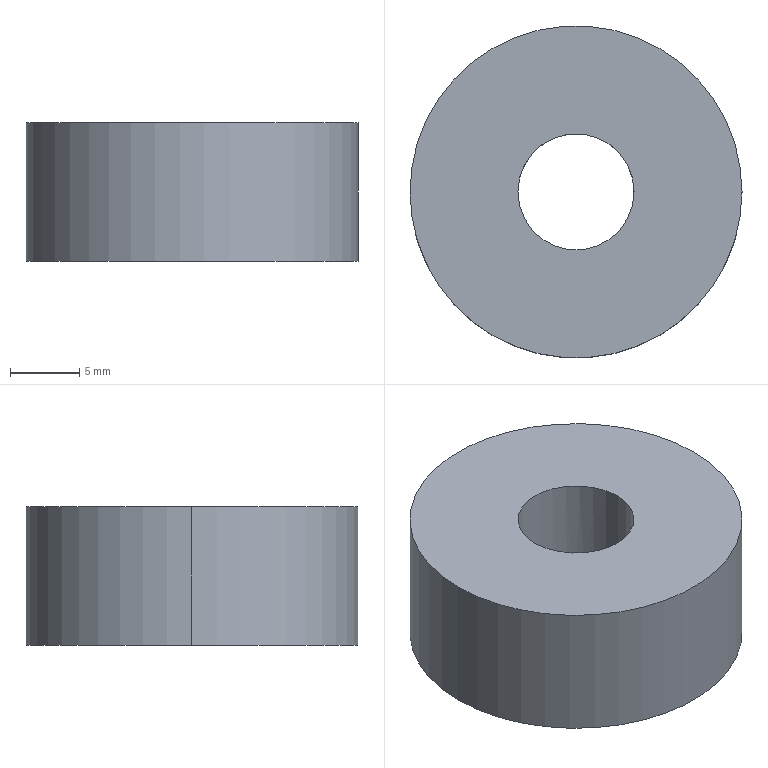Part | STEP file | PN_0033_Default<As Machined> | 1 solid | 6 faces | box 24 x 24 x 10 mm | volume 3970 mm3 | cylinder 4 | plane 2 | commonest cylinder face diameters 8.4 x2 24 x2
STEP:
#1=CARTESIAN_POINT('',(-4.2,0.,-10.));
#2=VERTEX_POINT('',#1);
#3=CARTESIAN_POINT('',(4.2,0.,-10.));
#4=VERTEX_POINT('',#3);
#5=CARTESIAN_POINT('',(0.,0.,-10.));
#6=DIRECTION('',(0.,0.,1.));
#7=AXIS2_PLACEMENT_3D('',#5,#6,$);
#8=CIRCLE('',#7,4.2);
#9=EDGE_CURVE('',#2,#4,#8,.T.);
#10=ORIENTED_EDGE('',*,*,#9,.F.);
#11=CARTESIAN_POINT('',(-4.2,0.,0.));
#12=VERTEX_POINT('',#11);
#13=CARTESIAN_POINT('',(-4.2,0.,-2.));
#14=DIRECTION('',(0.,0.,1.));
#15=VECTOR('',#14,1.);
#16=LINE('',#13,#15);
#17=EDGE_CURVE('',#2,#12,#16,.T.);
#18=ORIENTED_EDGE('',*,*,#17,.T.);
#19=CARTESIAN_POINT('',(4.2,0.,0.));
#20=VERTEX_POINT('',#19);
#21=CARTESIAN_POINT('',(0.,0.,0.));
#22=DIRECTION('',(0.,0.,1.));
#23=AXIS2_PLACEMENT_3D('',#21,#22,$);
#24=CIRCLE('',#23,4.2);
#25=EDGE_CURVE('',#12,#20,#24,.T.);
#26=ORIENTED_EDGE('',*,*,#25,.T.);
#27=CARTESIAN_POINT('',(4.2,0.,-2.));
#28=DIRECTION('',(0.,0.,1.));
#29=VECTOR('',#28,1.);
#30=LINE('',#27,#29);
#31=EDGE_CURVE('',#4,#20,#30,.T.);
#32=ORIENTED_EDGE('',*,*,#31,.F.);
#33=EDGE_LOOP('',(#10,#18,#26,#32));
#34=FACE_OUTER_BOUND('',#33,.T.);
#35=CARTESIAN_POINT('',(0.,0.,-2.));
#36=DIRECTION('',(0.,0.,1.));
#37=DIRECTION('',(-1.,0.,0.));
#38=AXIS2_PLACEMENT_3D('',#35,#36,#37);
#39=CYLINDRICAL_SURFACE('',#38,4.2);
#40=ADVANCED_FACE('',(#34),#39,.F.);
#41=CARTESIAN_POINT('',(12.,0.,-10.));
#42=VERTEX_POINT('',#41);
#43=CARTESIAN_POINT('',(-12.,0.,-10.));
#44=VERTEX_POINT('',#43);
#45=CARTESIAN_POINT('',(0.,0.,-10.));
#46=DIRECTION('',(0.,0.,-1.));
#47=AXIS2_PLACEMENT_3D('',#45,#46,$);
#48=CIRCLE('',#47,12.);
#49=EDGE_CURVE('',#42,#44,#48,.T.);
#50=ORIENTED_EDGE('',*,*,#49,.T.);
#51=CARTESIAN_POINT('',(0.,0.,-10.));
#52=DIRECTION('',(0.,0.,-1.));
#53=AXIS2_PLACEMENT_3D('',#51,#52,$);
#54=CIRCLE('',#53,12.);
#55=EDGE_CURVE('',#44,#42,#54,.T.);
#56=ORIENTED_EDGE('',*,*,#55,.T.);
#57=EDGE_LOOP('',(#50,#56));
#58=FACE_OUTER_BOUND('',#57,.T.);
#59=CARTESIAN_POINT('',(4.2,0.,-10.));
#60=CARTESIAN_POINT('',(4.2,0.4016,-10.));
#61=CARTESIAN_POINT('',(4.152,0.8032,-10.));
#62=CARTESIAN_POINT('',(4.056,1.197,-10.));
#63=CARTESIAN_POINT('',(3.772,1.954,-10.));
#64=CARTESIAN_POINT('',(3.317,2.623,-10.));
#65=CARTESIAN_POINT('',(3.05,2.929,-10.));
#66=CARTESIAN_POINT('',(2.45,3.471,-10.));
#67=CARTESIAN_POINT('',(1.738,3.855,-10.));
#68=CARTESIAN_POINT('',(1.361,4.004,-10.));
#69=CARTESIAN_POINT('',(0.5781,4.208,-10.));
#70=CARTESIAN_POINT('',(-0.2306,4.223,-10.));
#71=CARTESIAN_POINT('',(-0.634,4.181,-10.));
#72=CARTESIAN_POINT('',(-1.423,4.003,-10.));
#73=CARTESIAN_POINT('',(-2.148,3.643,-10.));
#74=CARTESIAN_POINT('',(-2.487,3.421,-10.));
#75=CARTESIAN_POINT('',(-3.105,2.899,-10.));
#76=CARTESIAN_POINT('',(-3.583,2.247,-10.));
#77=CARTESIAN_POINT('',(-3.782,1.893,-10.));
#78=CARTESIAN_POINT('',(-4.024,1.306,-10.));
#79=CARTESIAN_POINT('',(-4.153,0.6866,-10.));
#80=CARTESIAN_POINT('',(-4.184,0.4587,-10.));
#81=CARTESIAN_POINT('',(-4.2,0.2294,-10.));
#82=CARTESIAN_POINT('',(-4.2,0.,-10.));
#83=B_SPLINE_CURVE_WITH_KNOTS('',5,(#59,#60,#61,#62,#63,#64,#65,#66,#67,#68,#69,#70,#71,#72,#73,#74,#75,#76,#77,#78,#79,#80,#81,#82),.UNSPECIFIED.,.F.,.U.,(6,3,3,3,3,3,3,6),(0.,2.84,5.679,8.519,11.359,14.198,17.038,18.66),.UNSPECIFIED.);
#84=EDGE_CURVE('',#4,#2,#83,.T.);
#85=ORIENTED_EDGE('',*,*,#84,.T.);
#86=ORIENTED_EDGE('',*,*,#9,.T.);
#87=EDGE_LOOP('',(#85,#86));
#88=FACE_BOUND('',#87,.T.);
#89=CARTESIAN_POINT('',(0.,0.,-10.));
#90=DIRECTION('',(0.,0.,-1.));
#91=DIRECTION('',(-1.,0.,0.));
#92=AXIS2_PLACEMENT_3D('',#89,#90,#91);
#93=PLANE('',#92);
#94=ADVANCED_FACE('',(#58,#88),#93,.T.);
#95=ORIENTED_EDGE('',*,*,#17,.F.);
#96=ORIENTED_EDGE('',*,*,#84,.F.);
#97=ORIENTED_EDGE('',*,*,#31,.T.);
#98=CARTESIAN_POINT('',(0.,0.,0.));
#99=DIRECTION('',(0.,0.,1.));
#100=AXIS2_PLACEMENT_3D('',#98,#99,$);
#101=CIRCLE('',#100,4.2);
#102=EDGE_CURVE('',#20,#12,#101,.T.);
#103=ORIENTED_EDGE('',*,*,#102,.T.);
#104=EDGE_LOOP('',(#95,#96,#97,#103));
#105=FACE_OUTER_BOUND('',#104,.T.);
#106=CARTESIAN_POINT('',(0.,0.,-2.));
#107=DIRECTION('',(0.,0.,1.));
#108=DIRECTION('',(1.,0.,0.));
#109=AXIS2_PLACEMENT_3D('',#106,#107,#108);
#110=CYLINDRICAL_SURFACE('',#109,4.2);
#111=ADVANCED_FACE('',(#105),#110,.F.);
#112=CARTESIAN_POINT('',(12.,0.,0.));
#113=VERTEX_POINT('',#112);
#114=CARTESIAN_POINT('',(-12.,0.,0.));
#115=VERTEX_POINT('',#114);
#116=CARTESIAN_POINT('',(0.,0.,0.));
#117=DIRECTION('',(0.,0.,1.));
#118=AXIS2_PLACEMENT_3D('',#116,#117,$);
#119=CIRCLE('',#118,12.);
#120=EDGE_CURVE('',#113,#115,#119,.T.);
#121=ORIENTED_EDGE('',*,*,#120,.T.);
#122=CARTESIAN_POINT('',(0.,0.,0.));
#123=DIRECTION('',(0.,0.,1.));
#124=AXIS2_PLACEMENT_3D('',#122,#123,$);
#125=CIRCLE('',#124,12.);
#126=EDGE_CURVE('',#115,#113,#125,.T.);
#127=ORIENTED_EDGE('',*,*,#126,.T.);
#128=EDGE_LOOP('',(#121,#127));
#129=FACE_OUTER_BOUND('',#128,.T.);
#130=ORIENTED_EDGE('',*,*,#102,.F.);
#131=ORIENTED_EDGE('',*,*,#25,.F.);
#132=EDGE_LOOP('',(#130,#131));
#133=FACE_BOUND('',#132,.T.);
#134=CARTESIAN_POINT('',(0.,0.,0.));
#135=DIRECTION('',(0.,0.,1.));
#136=DIRECTION('',(1.,0.,0.));
#137=AXIS2_PLACEMENT_3D('',#134,#135,#136);
#138=PLANE('',#137);
#139=ADVANCED_FACE('',(#129,#133),#138,.T.);
#140=CARTESIAN_POINT('',(-12.,0.,-2.));
#141=DIRECTION('',(0.,0.,1.));
#142=VECTOR('',#141,1.);
#143=LINE('',#140,#142);
#144=EDGE_CURVE('',#44,#115,#143,.T.);
#145=ORIENTED_EDGE('',*,*,#144,.F.);
#146=ORIENTED_EDGE('',*,*,#49,.F.);
#147=CARTESIAN_POINT('',(12.,0.,-2.));
#148=DIRECTION('',(0.,0.,1.));
#149=VECTOR('',#148,1.);
#150=LINE('',#147,#149);
#151=EDGE_CURVE('',#42,#113,#150,.T.);
#152=ORIENTED_EDGE('',*,*,#151,.T.);
#153=ORIENTED_EDGE('',*,*,#126,.F.);
#154=EDGE_LOOP('',(#145,#146,#152,#153));
#155=FACE_OUTER_BOUND('',#154,.T.);
#156=CARTESIAN_POINT('',(0.,0.,-2.));
#157=DIRECTION('',(0.,0.,1.));
#158=DIRECTION('',(-1.,0.,0.));
#159=AXIS2_PLACEMENT_3D('',#156,#157,#158);
#160=CYLINDRICAL_SURFACE('',#159,12.);
#161=ADVANCED_FACE('',(#155),#160,.T.);
#162=ORIENTED_EDGE('',*,*,#55,.F.);
#163=ORIENTED_EDGE('',*,*,#144,.T.);
#164=ORIENTED_EDGE('',*,*,#120,.F.);
#165=ORIENTED_EDGE('',*,*,#151,.F.);
#166=EDGE_LOOP('',(#162,#163,#164,#165));
#167=FACE_OUTER_BOUND('',#166,.T.);
#168=CARTESIAN_POINT('',(0.,0.,-2.));
#169=DIRECTION('',(0.,0.,1.));
#170=DIRECTION('',(1.,0.,0.));
#171=AXIS2_PLACEMENT_3D('',#168,#169,#170);
#172=CYLINDRICAL_SURFACE('',#171,12.);
#173=ADVANCED_FACE('',(#167),#172,.T.);
#174=CLOSED_SHELL('',(#40,#94,#111,#139,#161,#173));
#175=MANIFOLD_SOLID_BREP('',#174);
#176=(LENGTH_UNIT()NAMED_UNIT(*)SI_UNIT(.MILLI.,.METRE.));
#177=UNCERTAINTY_MEASURE_WITH_UNIT(LENGTH_MEASURE(0.005),#176,'','');
#178=(NAMED_UNIT(*)PLANE_ANGLE_UNIT()SI_UNIT($,.RADIAN.));
#179=(NAMED_UNIT(*)SI_UNIT($,.STERADIAN.)SOLID_ANGLE_UNIT());
#180=(GEOMETRIC_REPRESENTATION_CONTEXT(3)GLOBAL_UNCERTAINTY_ASSIGNED_CONTEXT((#177))GLOBAL_UNIT_ASSIGNED_CONTEXT((#176,#178,#179))REPRESENTATION_CONTEXT('',''));
#181=ADVANCED_BREP_SHAPE_REPRESENTATION('',(#175),#180);